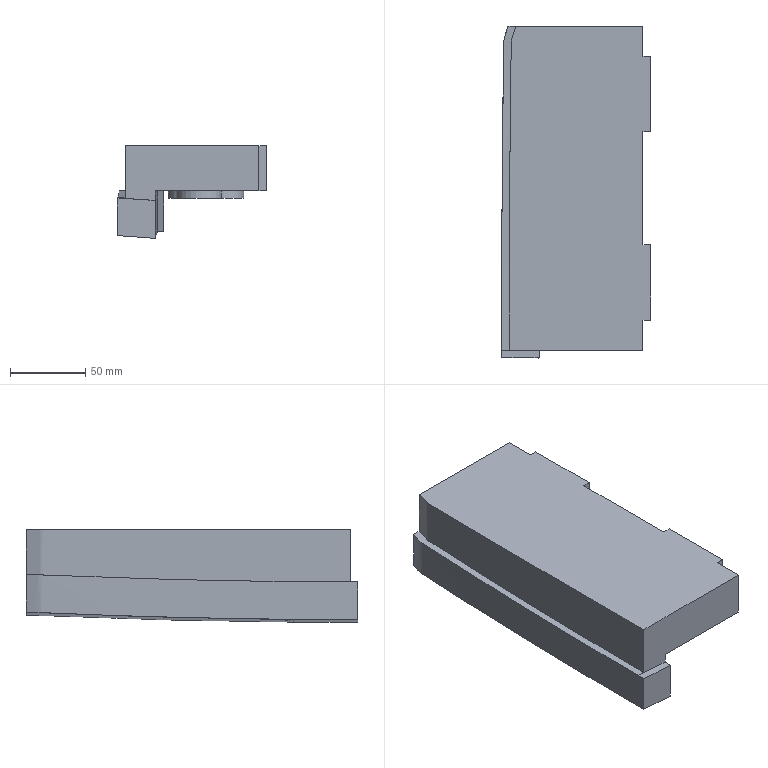Part | NX | features solid 2 | 1 solid | 33 faces | box 98.803 x 220 x 61.493 mm | volume 760096 mm3 | plane 18 | spline 10 | cylinder 5 | commonest cylinder face diameters 30 x5